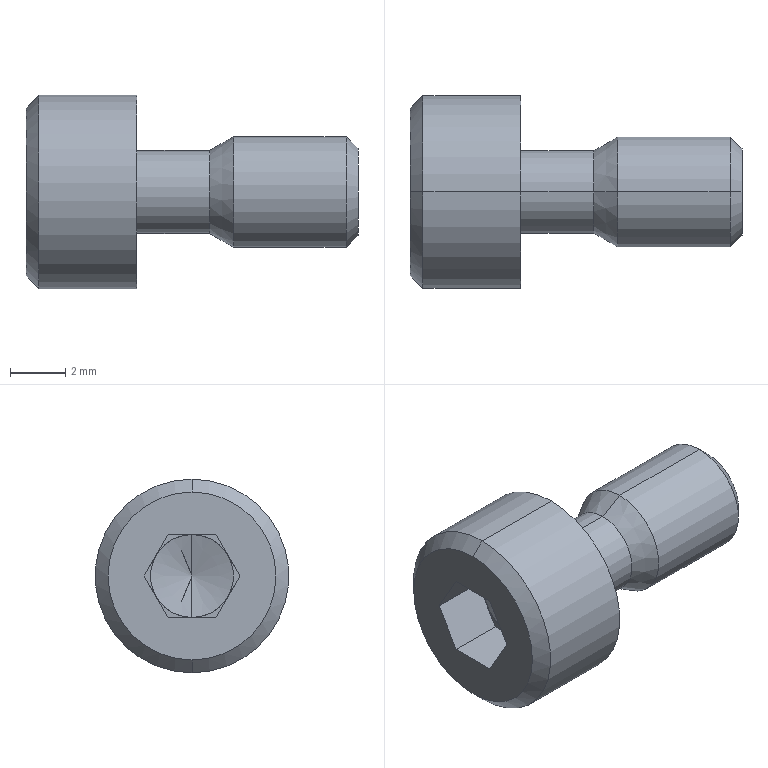Part | STEP file | 0243_Z_SCBZ4-8_1 | 1 solid | 31 faces | box 12 x 7 x 7 mm | volume 217.563 mm3 | plane 15 | cylinder 8 | cone 8 | commonest cylinder face diameters 3 x4 4 x2 7 x2